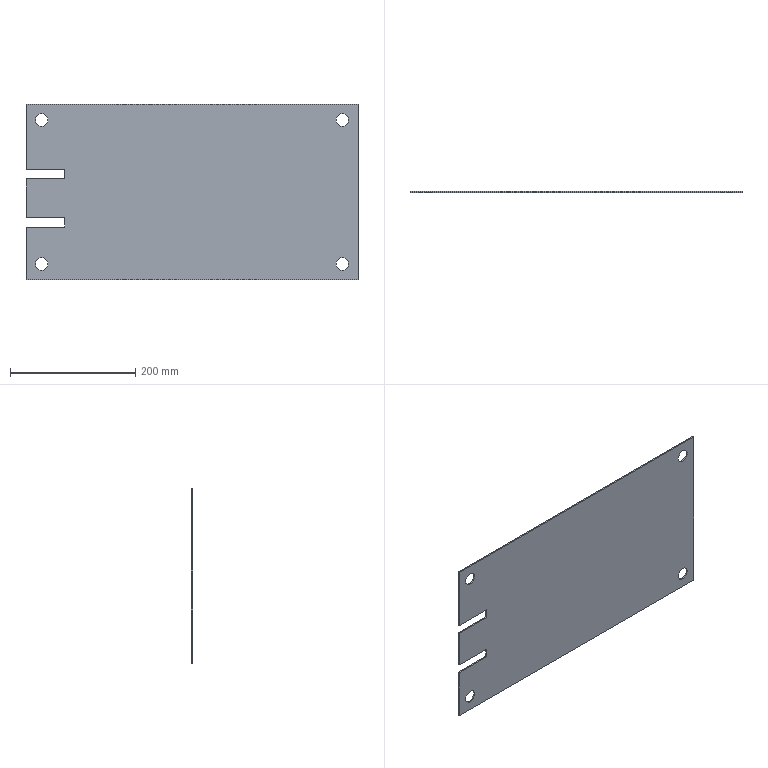Part | SolidWorks | features ICE 2, Extrusion 1 | 1 solid | 22 faces | box 530 x 2 x 280 mm | volume 290567 mm3 | plane 14 | cylinder 8 | commonest cylinder face diameters 20 x8
STEP:
#1=CARTESIAN_POINT('',(240.,0.,-125.));
#2=VERTEX_POINT('',#1);
#3=CARTESIAN_POINT('',(240.,0.,-105.));
#4=VERTEX_POINT('',#3);
#5=CARTESIAN_POINT('',(240.,0.,-115.));
#6=DIRECTION('',(0.,1.,0.));
#7=DIRECTION('',(0.,0.,-1.));
#8=AXIS2_PLACEMENT_3D('',#5,#6,#7);
#9=CIRCLE('',#8,10.);
#10=EDGE_CURVE('',#2,#4,#9,.T.);
#11=ORIENTED_EDGE('',*,*,#10,.F.);
#12=CARTESIAN_POINT('',(240.,2.,-125.));
#13=VERTEX_POINT('',#12);
#14=CARTESIAN_POINT('',(240.,0.,-125.));
#15=DIRECTION('',(0.,1.,0.));
#16=VECTOR('',#15,1000.);
#17=LINE('',#14,#16);
#18=EDGE_CURVE('',#2,#13,#17,.T.);
#19=ORIENTED_EDGE('',*,*,#18,.T.);
#20=CARTESIAN_POINT('',(240.,2.,-105.));
#21=VERTEX_POINT('',#20);
#22=CARTESIAN_POINT('',(240.,2.,-115.));
#23=DIRECTION('',(0.,1.,0.));
#24=DIRECTION('',(0.,0.,-1.));
#25=AXIS2_PLACEMENT_3D('',#22,#23,#24);
#26=CIRCLE('',#25,10.);
#27=EDGE_CURVE('',#13,#21,#26,.T.);
#28=ORIENTED_EDGE('',*,*,#27,.T.);
#29=CARTESIAN_POINT('',(240.,0.,-105.));
#30=DIRECTION('',(0.,1.,0.));
#31=VECTOR('',#30,1000.);
#32=LINE('',#29,#31);
#33=EDGE_CURVE('',#4,#21,#32,.T.);
#34=ORIENTED_EDGE('',*,*,#33,.F.);
#35=EDGE_LOOP('',(#11,#19,#28,#34));
#36=FACE_OUTER_BOUND('',#35,.T.);
#37=CARTESIAN_POINT('',(240.,0.,-115.));
#38=DIRECTION('',(0.,1.,0.));
#39=DIRECTION('',(0.,0.,1.));
#40=AXIS2_PLACEMENT_3D('',#37,#38,#39);
#41=CYLINDRICAL_SURFACE('',#40,10.);
#42=ADVANCED_FACE('',(#36),#41,.F.);
#43=CARTESIAN_POINT('',(240.,0.,105.));
#44=VERTEX_POINT('',#43);
#45=CARTESIAN_POINT('',(240.,0.,125.));
#46=VERTEX_POINT('',#45);
#47=CARTESIAN_POINT('',(240.,0.,115.));
#48=DIRECTION('',(0.,1.,0.));
#49=DIRECTION('',(0.,0.,1.));
#50=AXIS2_PLACEMENT_3D('',#47,#48,#49);
#51=CIRCLE('',#50,10.);
#52=EDGE_CURVE('',#44,#46,#51,.T.);
#53=ORIENTED_EDGE('',*,*,#52,.F.);
#54=CARTESIAN_POINT('',(240.,2.,105.));
#55=VERTEX_POINT('',#54);
#56=CARTESIAN_POINT('',(240.,0.,105.));
#57=DIRECTION('',(0.,1.,0.));
#58=VECTOR('',#57,1000.);
#59=LINE('',#56,#58);
#60=EDGE_CURVE('',#44,#55,#59,.T.);
#61=ORIENTED_EDGE('',*,*,#60,.T.);
#62=CARTESIAN_POINT('',(240.,2.,125.));
#63=VERTEX_POINT('',#62);
#64=CARTESIAN_POINT('',(240.,2.,115.));
#65=DIRECTION('',(0.,1.,0.));
#66=DIRECTION('',(0.,0.,1.));
#67=AXIS2_PLACEMENT_3D('',#64,#65,#66);
#68=CIRCLE('',#67,10.);
#69=EDGE_CURVE('',#55,#63,#68,.T.);
#70=ORIENTED_EDGE('',*,*,#69,.T.);
#71=CARTESIAN_POINT('',(240.,0.,125.));
#72=DIRECTION('',(0.,1.,0.));
#73=VECTOR('',#72,1000.);
#74=LINE('',#71,#73);
#75=EDGE_CURVE('',#46,#63,#74,.T.);
#76=ORIENTED_EDGE('',*,*,#75,.F.);
#77=EDGE_LOOP('',(#53,#61,#70,#76));
#78=FACE_OUTER_BOUND('',#77,.T.);
#79=CARTESIAN_POINT('',(240.,0.,115.));
#80=DIRECTION('',(0.,1.,0.));
#81=DIRECTION('',(0.,0.,1.));
#82=AXIS2_PLACEMENT_3D('',#79,#80,#81);
#83=CYLINDRICAL_SURFACE('',#82,10.);
#84=ADVANCED_FACE('',(#78),#83,.F.);
#85=CARTESIAN_POINT('',(-240.,0.,105.));
#86=VERTEX_POINT('',#85);
#87=CARTESIAN_POINT('',(-240.,0.,125.));
#88=VERTEX_POINT('',#87);
#89=CARTESIAN_POINT('',(-240.,0.,115.));
#90=DIRECTION('',(0.,1.,0.));
#91=DIRECTION('',(0.,0.,-1.));
#92=AXIS2_PLACEMENT_3D('',#89,#90,#91);
#93=CIRCLE('',#92,10.);
#94=EDGE_CURVE('',#86,#88,#93,.T.);
#95=ORIENTED_EDGE('',*,*,#94,.F.);
#96=CARTESIAN_POINT('',(-240.,2.,105.));
#97=VERTEX_POINT('',#96);
#98=CARTESIAN_POINT('',(-240.,0.,105.));
#99=DIRECTION('',(0.,1.,0.));
#100=VECTOR('',#99,1000.);
#101=LINE('',#98,#100);
#102=EDGE_CURVE('',#86,#97,#101,.T.);
#103=ORIENTED_EDGE('',*,*,#102,.T.);
#104=CARTESIAN_POINT('',(-240.,2.,125.));
#105=VERTEX_POINT('',#104);
#106=CARTESIAN_POINT('',(-240.,2.,115.));
#107=DIRECTION('',(0.,1.,0.));
#108=DIRECTION('',(0.,0.,-1.));
#109=AXIS2_PLACEMENT_3D('',#106,#107,#108);
#110=CIRCLE('',#109,10.);
#111=EDGE_CURVE('',#97,#105,#110,.T.);
#112=ORIENTED_EDGE('',*,*,#111,.T.);
#113=CARTESIAN_POINT('',(-240.,0.,125.));
#114=DIRECTION('',(0.,1.,0.));
#115=VECTOR('',#114,1000.);
#116=LINE('',#113,#115);
#117=EDGE_CURVE('',#88,#105,#116,.T.);
#118=ORIENTED_EDGE('',*,*,#117,.F.);
#119=EDGE_LOOP('',(#95,#103,#112,#118));
#120=FACE_OUTER_BOUND('',#119,.T.);
#121=CARTESIAN_POINT('',(-240.,0.,115.));
#122=DIRECTION('',(0.,1.,0.));
#123=DIRECTION('',(0.,0.,1.));
#124=AXIS2_PLACEMENT_3D('',#121,#122,#123);
#125=CYLINDRICAL_SURFACE('',#124,10.);
#126=ADVANCED_FACE('',(#120),#125,.F.);
#127=CARTESIAN_POINT('',(-240.,0.,-125.));
#128=VERTEX_POINT('',#127);
#129=CARTESIAN_POINT('',(-240.,0.,-105.));
#130=VERTEX_POINT('',#129);
#131=CARTESIAN_POINT('',(-240.,0.,-115.));
#132=DIRECTION('',(0.,1.,0.));
#133=DIRECTION('',(0.,0.,1.));
#134=AXIS2_PLACEMENT_3D('',#131,#132,#133);
#135=CIRCLE('',#134,10.);
#136=EDGE_CURVE('',#128,#130,#135,.T.);
#137=ORIENTED_EDGE('',*,*,#136,.F.);
#138=CARTESIAN_POINT('',(-240.,2.,-125.));
#139=VERTEX_POINT('',#138);
#140=CARTESIAN_POINT('',(-240.,0.,-125.));
#141=DIRECTION('',(0.,1.,0.));
#142=VECTOR('',#141,1000.);
#143=LINE('',#140,#142);
#144=EDGE_CURVE('',#128,#139,#143,.T.);
#145=ORIENTED_EDGE('',*,*,#144,.T.);
#146=CARTESIAN_POINT('',(-240.,2.,-105.));
#147=VERTEX_POINT('',#146);
#148=CARTESIAN_POINT('',(-240.,2.,-115.));
#149=DIRECTION('',(0.,1.,0.));
#150=DIRECTION('',(0.,0.,1.));
#151=AXIS2_PLACEMENT_3D('',#148,#149,#150);
#152=CIRCLE('',#151,10.);
#153=EDGE_CURVE('',#139,#147,#152,.T.);
#154=ORIENTED_EDGE('',*,*,#153,.T.);
#155=CARTESIAN_POINT('',(-240.,0.,-105.));
#156=DIRECTION('',(0.,1.,0.));
#157=VECTOR('',#156,1000.);
#158=LINE('',#155,#157);
#159=EDGE_CURVE('',#130,#147,#158,.T.);
#160=ORIENTED_EDGE('',*,*,#159,.F.);
#161=EDGE_LOOP('',(#137,#145,#154,#160));
#162=FACE_OUTER_BOUND('',#161,.T.);
#163=CARTESIAN_POINT('',(-240.,0.,-115.));
#164=DIRECTION('',(0.,1.,0.));
#165=DIRECTION('',(0.,0.,1.));
#166=AXIS2_PLACEMENT_3D('',#163,#164,#165);
#167=CYLINDRICAL_SURFACE('',#166,10.);
#168=ADVANCED_FACE('',(#162),#167,.F.);
#169=CARTESIAN_POINT('',(-265.,0.,-41.));
#170=VERTEX_POINT('',#169);
#171=CARTESIAN_POINT('',(-265.,0.,21.));
#172=VERTEX_POINT('',#171);
#173=CARTESIAN_POINT('',(-265.,0.,140.));
#174=DIRECTION('',(0.,0.,1.));
#175=VECTOR('',#174,1000.);
#176=LINE('',#173,#175);
#177=EDGE_CURVE('',#170,#172,#176,.T.);
#178=ORIENTED_EDGE('',*,*,#177,.T.);
#179=CARTESIAN_POINT('',(-265.,2.,21.));
#180=VERTEX_POINT('',#179);
#181=CARTESIAN_POINT('',(-265.,2.,21.));
#182=DIRECTION('',(0.,1.,0.));
#183=VECTOR('',#182,1000.);
#184=LINE('',#181,#183);
#185=EDGE_CURVE('',#172,#180,#184,.T.);
#186=ORIENTED_EDGE('',*,*,#185,.T.);
#187=CARTESIAN_POINT('',(-265.,2.,-41.));
#188=VERTEX_POINT('',#187);
#189=CARTESIAN_POINT('',(-265.,2.,140.));
#190=DIRECTION('',(0.,0.,1.));
#191=VECTOR('',#190,1000.);
#192=LINE('',#189,#191);
#193=EDGE_CURVE('',#188,#180,#192,.T.);
#194=ORIENTED_EDGE('',*,*,#193,.F.);
#195=CARTESIAN_POINT('',(-265.,2.,-41.));
#196=DIRECTION('',(0.,-1.,0.));
#197=VECTOR('',#196,1000.);
#198=LINE('',#195,#197);
#199=EDGE_CURVE('',#188,#170,#198,.T.);
#200=ORIENTED_EDGE('',*,*,#199,.T.);
#201=EDGE_LOOP('',(#178,#186,#194,#200));
#202=FACE_OUTER_BOUND('',#201,.T.);
#203=CARTESIAN_POINT('',(-265.,2.,140.));
#204=DIRECTION('',(1.,0.,0.));
#205=DIRECTION('',(0.,0.,-1.));
#206=AXIS2_PLACEMENT_3D('',#203,#204,#205);
#207=PLANE('',#206);
#208=ADVANCED_FACE('',(#202),#207,.F.);
#209=CARTESIAN_POINT('',(-265.,0.,-140.));
#210=VERTEX_POINT('',#209);
#211=CARTESIAN_POINT('',(-265.,0.,-56.));
#212=VERTEX_POINT('',#211);
#213=CARTESIAN_POINT('',(-265.,0.,140.));
#214=DIRECTION('',(0.,0.,1.));
#215=VECTOR('',#214,1000.);
#216=LINE('',#213,#215);
#217=EDGE_CURVE('',#210,#212,#216,.T.);
#218=ORIENTED_EDGE('',*,*,#217,.T.);
#219=CARTESIAN_POINT('',(-265.,2.,-56.));
#220=VERTEX_POINT('',#219);
#221=CARTESIAN_POINT('',(-265.,2.,-56.));
#222=DIRECTION('',(0.,1.,0.));
#223=VECTOR('',#222,1000.);
#224=LINE('',#221,#223);
#225=EDGE_CURVE('',#212,#220,#224,.T.);
#226=ORIENTED_EDGE('',*,*,#225,.T.);
#227=CARTESIAN_POINT('',(-265.,2.,-140.));
#228=VERTEX_POINT('',#227);
#229=CARTESIAN_POINT('',(-265.,2.,140.));
#230=DIRECTION('',(0.,0.,1.));
#231=VECTOR('',#230,1000.);
#232=LINE('',#229,#231);
#233=EDGE_CURVE('',#228,#220,#232,.T.);
#234=ORIENTED_EDGE('',*,*,#233,.F.);
#235=CARTESIAN_POINT('',(-265.,2.,-140.));
#236=DIRECTION('',(0.,-1.,0.));
#237=VECTOR('',#236,1000.);
#238=LINE('',#235,#237);
#239=EDGE_CURVE('',#228,#210,#238,.T.);
#240=ORIENTED_EDGE('',*,*,#239,.T.);
#241=EDGE_LOOP('',(#218,#226,#234,#240));
#242=FACE_OUTER_BOUND('',#241,.T.);
#243=CARTESIAN_POINT('',(-265.,2.,140.));
#244=DIRECTION('',(1.,0.,0.));
#245=DIRECTION('',(0.,0.,-1.));
#246=AXIS2_PLACEMENT_3D('',#243,#244,#245);
#247=PLANE('',#246);
#248=ADVANCED_FACE('',(#242),#247,.F.);
#249=CARTESIAN_POINT('',(265.,0.,140.));
#250=VERTEX_POINT('',#249);
#251=CARTESIAN_POINT('',(265.,0.,-140.));
#252=VERTEX_POINT('',#251);
#253=CARTESIAN_POINT('',(265.,0.,140.));
#254=DIRECTION('',(0.,0.,-1.));
#255=VECTOR('',#254,1000.);
#256=LINE('',#253,#255);
#257=EDGE_CURVE('',#250,#252,#256,.T.);
#258=ORIENTED_EDGE('',*,*,#257,.T.);
#259=CARTESIAN_POINT('',(265.,2.,-140.));
#260=VERTEX_POINT('',#259);
#261=CARTESIAN_POINT('',(265.,2.,-140.));
#262=DIRECTION('',(0.,-1.,0.));
#263=VECTOR('',#262,1000.);
#264=LINE('',#261,#263);
#265=EDGE_CURVE('',#260,#252,#264,.T.);
#266=ORIENTED_EDGE('',*,*,#265,.F.);
#267=CARTESIAN_POINT('',(265.,2.,140.));
#268=VERTEX_POINT('',#267);
#269=CARTESIAN_POINT('',(265.,2.,140.));
#270=DIRECTION('',(0.,0.,-1.));
#271=VECTOR('',#270,1000.);
#272=LINE('',#269,#271);
#273=EDGE_CURVE('',#268,#260,#272,.T.);
#274=ORIENTED_EDGE('',*,*,#273,.F.);
#275=CARTESIAN_POINT('',(265.,2.,140.));
#276=DIRECTION('',(0.,-1.,0.));
#277=VECTOR('',#276,1000.);
#278=LINE('',#275,#277);
#279=EDGE_CURVE('',#268,#250,#278,.T.);
#280=ORIENTED_EDGE('',*,*,#279,.T.);
#281=EDGE_LOOP('',(#258,#266,#274,#280));
#282=FACE_OUTER_BOUND('',#281,.T.);
#283=CARTESIAN_POINT('',(265.,2.,140.));
#284=DIRECTION('',(-1.,0.,0.));
#285=DIRECTION('',(0.,0.,1.));
#286=AXIS2_PLACEMENT_3D('',#283,#284,#285);
#287=PLANE('',#286);
#288=ADVANCED_FACE('',(#282),#287,.F.);
#289=CARTESIAN_POINT('',(-265.,0.,-140.));
#290=DIRECTION('',(-1.,0.,0.));
#291=VECTOR('',#290,1000.);
#292=LINE('',#289,#291);
#293=EDGE_CURVE('',#252,#210,#292,.T.);
#294=ORIENTED_EDGE('',*,*,#293,.T.);
#295=ORIENTED_EDGE('',*,*,#239,.F.);
#296=CARTESIAN_POINT('',(-265.,2.,-140.));
#297=DIRECTION('',(-1.,0.,0.));
#298=VECTOR('',#297,1000.);
#299=LINE('',#296,#298);
#300=EDGE_CURVE('',#260,#228,#299,.T.);
#301=ORIENTED_EDGE('',*,*,#300,.F.);
#302=ORIENTED_EDGE('',*,*,#265,.T.);
#303=EDGE_LOOP('',(#294,#295,#301,#302));
#304=FACE_OUTER_BOUND('',#303,.T.);
#305=CARTESIAN_POINT('',(-265.,2.,-140.));
#306=DIRECTION('',(0.,0.,1.));
#307=DIRECTION('',(1.,0.,0.));
#308=AXIS2_PLACEMENT_3D('',#305,#306,#307);
#309=PLANE('',#308);
#310=ADVANCED_FACE('',(#304),#309,.F.);
#311=CARTESIAN_POINT('',(-265.,2.,36.));
#312=VERTEX_POINT('',#311);
#313=CARTESIAN_POINT('',(-265.,2.,140.));
#314=VERTEX_POINT('',#313);
#315=CARTESIAN_POINT('',(-265.,2.,140.));
#316=DIRECTION('',(0.,0.,1.));
#317=VECTOR('',#316,1000.);
#318=LINE('',#315,#317);
#319=EDGE_CURVE('',#312,#314,#318,.T.);
#320=ORIENTED_EDGE('',*,*,#319,.F.);
#321=CARTESIAN_POINT('',(-265.,0.,36.));
#322=VERTEX_POINT('',#321);
#323=CARTESIAN_POINT('',(-265.,2.,36.));
#324=DIRECTION('',(0.,-1.,0.));
#325=VECTOR('',#324,1000.);
#326=LINE('',#323,#325);
#327=EDGE_CURVE('',#312,#322,#326,.T.);
#328=ORIENTED_EDGE('',*,*,#327,.T.);
#329=CARTESIAN_POINT('',(-265.,0.,140.));
#330=VERTEX_POINT('',#329);
#331=CARTESIAN_POINT('',(-265.,0.,140.));
#332=DIRECTION('',(0.,0.,1.));
#333=VECTOR('',#332,1000.);
#334=LINE('',#331,#333);
#335=EDGE_CURVE('',#322,#330,#334,.T.);
#336=ORIENTED_EDGE('',*,*,#335,.T.);
#337=CARTESIAN_POINT('',(-265.,2.,140.));
#338=DIRECTION('',(0.,-1.,0.));
#339=VECTOR('',#338,1000.);
#340=LINE('',#337,#339);
#341=EDGE_CURVE('',#314,#330,#340,.T.);
#342=ORIENTED_EDGE('',*,*,#341,.F.);
#343=EDGE_LOOP('',(#320,#328,#336,#342));
#344=FACE_OUTER_BOUND('',#343,.T.);
#345=CARTESIAN_POINT('',(-265.,2.,140.));
#346=DIRECTION('',(1.,0.,0.));
#347=DIRECTION('',(0.,0.,-1.));
#348=AXIS2_PLACEMENT_3D('',#345,#346,#347);
#349=PLANE('',#348);
#350=ADVANCED_FACE('',(#344),#349,.F.);
#351=CARTESIAN_POINT('',(-265.,0.,140.));
#352=DIRECTION('',(1.,0.,0.));
#353=VECTOR('',#352,1000.);
#354=LINE('',#351,#353);
#355=EDGE_CURVE('',#330,#250,#354,.T.);
#356=ORIENTED_EDGE('',*,*,#355,.T.);
#357=ORIENTED_EDGE('',*,*,#279,.F.);
#358=CARTESIAN_POINT('',(-265.,2.,140.));
#359=DIRECTION('',(1.,0.,0.));
#360=VECTOR('',#359,1000.);
#361=LINE('',#358,#360);
#362=EDGE_CURVE('',#314,#268,#361,.T.);
#363=ORIENTED_EDGE('',*,*,#362,.F.);
#364=ORIENTED_EDGE('',*,*,#341,.T.);
#365=EDGE_LOOP('',(#356,#357,#363,#364));
#366=FACE_OUTER_BOUND('',#365,.T.);
#367=CARTESIAN_POINT('',(-265.,2.,140.));
#368=DIRECTION('',(0.,0.,-1.));
#369=DIRECTION('',(-1.,0.,0.));
#370=AXIS2_PLACEMENT_3D('',#367,#368,#369);
#371=PLANE('',#370);
#372=ADVANCED_FACE('',(#366),#371,.F.);
#373=CARTESIAN_POINT('',(240.,2.,-115.));
#374=DIRECTION('',(0.,1.,0.));
#375=DIRECTION('',(0.,0.,-1.));
#376=AXIS2_PLACEMENT_3D('',#373,#374,#375);
#377=CIRCLE('',#376,10.);
#378=EDGE_CURVE('',#21,#13,#377,.T.);
#379=ORIENTED_EDGE('',*,*,#378,.F.);
#380=ORIENTED_EDGE('',*,*,#27,.F.);
#381=EDGE_LOOP('',(#379,#380));
#382=FACE_BOUND('',#381,.T.);
#383=CARTESIAN_POINT('',(240.,2.,115.));
#384=DIRECTION('',(0.,1.,0.));
#385=DIRECTION('',(0.,0.,1.));
#386=AXIS2_PLACEMENT_3D('',#383,#384,#385);
#387=CIRCLE('',#386,10.);
#388=EDGE_CURVE('',#63,#55,#387,.T.);
#389=ORIENTED_EDGE('',*,*,#388,.F.);
#390=ORIENTED_EDGE('',*,*,#69,.F.);
#391=EDGE_LOOP('',(#389,#390));
#392=FACE_BOUND('',#391,.T.);
#393=CARTESIAN_POINT('',(-240.,2.,115.));
#394=DIRECTION('',(0.,1.,0.));
#395=DIRECTION('',(0.,0.,-1.));
#396=AXIS2_PLACEMENT_3D('',#393,#394,#395);
#397=CIRCLE('',#396,10.);
#398=EDGE_CURVE('',#105,#97,#397,.T.);
#399=ORIENTED_EDGE('',*,*,#398,.F.);
#400=ORIENTED_EDGE('',*,*,#111,.F.);
#401=EDGE_LOOP('',(#399,#400));
#402=FACE_BOUND('',#401,.T.);
#403=CARTESIAN_POINT('',(-240.,2.,-115.));
#404=DIRECTION('',(0.,1.,0.));
#405=DIRECTION('',(0.,0.,1.));
#406=AXIS2_PLACEMENT_3D('',#403,#404,#405);
#407=CIRCLE('',#406,10.);
#408=EDGE_CURVE('',#147,#139,#407,.T.);
#409=ORIENTED_EDGE('',*,*,#408,.F.);
#410=ORIENTED_EDGE('',*,*,#153,.F.);
#411=EDGE_LOOP('',(#409,#410));
#412=FACE_BOUND('',#411,.T.);
#413=ORIENTED_EDGE('',*,*,#193,.T.);
#414=CARTESIAN_POINT('',(-203.,2.,21.));
#415=VERTEX_POINT('',#414);
#416=CARTESIAN_POINT('',(-299.084,2.,21.));
#417=DIRECTION('',(-1.,0.,0.));
#418=VECTOR('',#417,1000.);
#419=LINE('',#416,#418);
#420=EDGE_CURVE('',#415,#180,#419,.T.);
#421=ORIENTED_EDGE('',*,*,#420,.F.);
#422=CARTESIAN_POINT('',(-203.,2.,36.));
#423=VERTEX_POINT('',#422);
#424=CARTESIAN_POINT('',(-203.,2.,21.));
#425=DIRECTION('',(0.,0.,-1.));
#426=VECTOR('',#425,1000.);
#427=LINE('',#424,#426);
#428=EDGE_CURVE('',#423,#415,#427,.T.);
#429=ORIENTED_EDGE('',*,*,#428,.F.);
#430=CARTESIAN_POINT('',(-299.084,2.,36.));
#431=DIRECTION('',(1.,0.,0.));
#432=VECTOR('',#431,1000.);
#433=LINE('',#430,#432);
#434=EDGE_CURVE('',#312,#423,#433,.T.);
#435=ORIENTED_EDGE('',*,*,#434,.F.);
#436=ORIENTED_EDGE('',*,*,#319,.T.);
#437=ORIENTED_EDGE('',*,*,#362,.T.);
#438=ORIENTED_EDGE('',*,*,#273,.T.);
#439=ORIENTED_EDGE('',*,*,#300,.T.);
#440=ORIENTED_EDGE('',*,*,#233,.T.);
#441=CARTESIAN_POINT('',(-203.,2.,-56.));
#442=VERTEX_POINT('',#441);
#443=CARTESIAN_POINT('',(-296.313,2.,-56.));
#444=DIRECTION('',(-1.,0.,0.));
#445=VECTOR('',#444,1000.);
#446=LINE('',#443,#445);
#447=EDGE_CURVE('',#442,#220,#446,.T.);
#448=ORIENTED_EDGE('',*,*,#447,.F.);
#449=CARTESIAN_POINT('',(-203.,2.,-41.));
#450=VERTEX_POINT('',#449);
#451=CARTESIAN_POINT('',(-203.,2.,-56.));
#452=DIRECTION('',(0.,0.,-1.));
#453=VECTOR('',#452,1000.);
#454=LINE('',#451,#453);
#455=EDGE_CURVE('',#450,#442,#454,.T.);
#456=ORIENTED_EDGE('',*,*,#455,.F.);
#457=CARTESIAN_POINT('',(-296.313,2.,-41.));
#458=DIRECTION('',(1.,0.,0.));
#459=VECTOR('',#458,1000.);
#460=LINE('',#457,#459);
#461=EDGE_CURVE('',#188,#450,#460,.T.);
#462=ORIENTED_EDGE('',*,*,#461,.F.);
#463=EDGE_LOOP('',(#413,#421,#429,#435,#436,#437,#438,#439,#440,#448,#456,#462));
#464=FACE_OUTER_BOUND('',#463,.T.);
#465=CARTESIAN_POINT('',(0.,2.,0.));
#466=DIRECTION('',(0.,-1.,0.));
#467=DIRECTION('',(0.,0.,-1.));
#468=AXIS2_PLACEMENT_3D('',#465,#466,#467);
#469=PLANE('',#468);
#470=ADVANCED_FACE('',(#382,#392,#402,#412,#464),#469,.F.);
#471=CARTESIAN_POINT('',(-203.,0.,21.));
#472=VERTEX_POINT('',#471);
#473=CARTESIAN_POINT('',(0.,0.,21.));
#474=DIRECTION('',(1.,0.,0.));
#475=VECTOR('',#474,1000.);
#476=LINE('',#473,#475);
#477=EDGE_CURVE('',#172,#472,#476,.T.);
#478=ORIENTED_EDGE('',*,*,#477,.F.);
#479=ORIENTED_EDGE('',*,*,#177,.F.);
#480=CARTESIAN_POINT('',(-203.,0.,-41.));
#481=VERTEX_POINT('',#480);
#482=CARTESIAN_POINT('',(0.,0.,-41.));
#483=DIRECTION('',(-1.,0.,0.));
#484=VECTOR('',#483,1000.);
#485=LINE('',#482,#484);
#486=EDGE_CURVE('',#481,#170,#485,.T.);
#487=ORIENTED_EDGE('',*,*,#486,.F.);
#488=CARTESIAN_POINT('',(-203.,0.,-56.));
#489=VERTEX_POINT('',#488);
#490=CARTESIAN_POINT('',(-203.,0.,0.));
#491=DIRECTION('',(0.,0.,1.));
#492=VECTOR('',#491,1000.);
#493=LINE('',#490,#492);
#494=EDGE_CURVE('',#489,#481,#493,.T.);
#495=ORIENTED_EDGE('',*,*,#494,.F.);
#496=CARTESIAN_POINT('',(0.,0.,-56.));
#497=DIRECTION('',(1.,0.,0.));
#498=VECTOR('',#497,1000.);
#499=LINE('',#496,#498);
#500=EDGE_CURVE('',#212,#489,#499,.T.);
#501=ORIENTED_EDGE('',*,*,#500,.F.);
#502=ORIENTED_EDGE('',*,*,#217,.F.);
#503=ORIENTED_EDGE('',*,*,#293,.F.);
#504=ORIENTED_EDGE('',*,*,#257,.F.);
#505=ORIENTED_EDGE('',*,*,#355,.F.);
#506=ORIENTED_EDGE('',*,*,#335,.F.);
#507=CARTESIAN_POINT('',(-203.,0.,36.));
#508=VERTEX_POINT('',#507);
#509=CARTESIAN_POINT('',(0.,0.,36.));
#510=DIRECTION('',(-1.,0.,0.));
#511=VECTOR('',#510,1000.);
#512=LINE('',#509,#511);
#513=EDGE_CURVE('',#508,#322,#512,.T.);
#514=ORIENTED_EDGE('',*,*,#513,.F.);
#515=CARTESIAN_POINT('',(-203.,0.,0.));
#516=DIRECTION('',(0.,0.,1.));
#517=VECTOR('',#516,1000.);
#518=LINE('',#515,#517);
#519=EDGE_CURVE('',#472,#508,#518,.T.);
#520=ORIENTED_EDGE('',*,*,#519,.F.);
#521=EDGE_LOOP('',(#478,#479,#487,#495,#501,#502,#503,#504,#505,#506,#514,#520));
#522=FACE_OUTER_BOUND('',#521,.T.);
#523=CARTESIAN_POINT('',(240.,0.,-115.));
#524=DIRECTION('',(0.,1.,0.));
#525=DIRECTION('',(0.,0.,-1.));
#526=AXIS2_PLACEMENT_3D('',#523,#524,#525);
#527=CIRCLE('',#526,10.);
#528=EDGE_CURVE('',#4,#2,#527,.T.);
#529=ORIENTED_EDGE('',*,*,#528,.T.);
#530=ORIENTED_EDGE('',*,*,#10,.T.);
#531=EDGE_LOOP('',(#529,#530));
#532=FACE_BOUND('',#531,.T.);
#533=CARTESIAN_POINT('',(240.,0.,115.));
#534=DIRECTION('',(0.,1.,0.));
#535=DIRECTION('',(0.,0.,1.));
#536=AXIS2_PLACEMENT_3D('',#533,#534,#535);
#537=CIRCLE('',#536,10.);
#538=EDGE_CURVE('',#46,#44,#537,.T.);
#539=ORIENTED_EDGE('',*,*,#538,.T.);
#540=ORIENTED_EDGE('',*,*,#52,.T.);
#541=EDGE_LOOP('',(#539,#540));
#542=FACE_BOUND('',#541,.T.);
#543=CARTESIAN_POINT('',(-240.,0.,115.));
#544=DIRECTION('',(0.,1.,0.));
#545=DIRECTION('',(0.,0.,-1.));
#546=AXIS2_PLACEMENT_3D('',#543,#544,#545);
#547=CIRCLE('',#546,10.);
#548=EDGE_CURVE('',#88,#86,#547,.T.);
#549=ORIENTED_EDGE('',*,*,#548,.T.);
#550=ORIENTED_EDGE('',*,*,#94,.T.);
#551=EDGE_LOOP('',(#549,#550));
#552=FACE_BOUND('',#551,.T.);
#553=CARTESIAN_POINT('',(-240.,0.,-115.));
#554=DIRECTION('',(0.,1.,0.));
#555=DIRECTION('',(0.,0.,1.));
#556=AXIS2_PLACEMENT_3D('',#553,#554,#555);
#557=CIRCLE('',#556,10.);
#558=EDGE_CURVE('',#130,#128,#557,.T.);
#559=ORIENTED_EDGE('',*,*,#558,.T.);
#560=ORIENTED_EDGE('',*,*,#136,.T.);
#561=EDGE_LOOP('',(#559,#560));
#562=FACE_BOUND('',#561,.T.);
#563=CARTESIAN_POINT('',(0.,0.,0.));
#564=DIRECTION('',(0.,-1.,0.));
#565=DIRECTION('',(0.,0.,-1.));
#566=AXIS2_PLACEMENT_3D('',#563,#564,#565);
#567=PLANE('',#566);
#568=ADVANCED_FACE('',(#522,#532,#542,#552,#562),#567,.T.);
#569=ORIENTED_EDGE('',*,*,#144,.F.);
#570=ORIENTED_EDGE('',*,*,#558,.F.);
#571=ORIENTED_EDGE('',*,*,#159,.T.);
#572=ORIENTED_EDGE('',*,*,#408,.T.);
#573=EDGE_LOOP('',(#569,#570,#571,#572));
#574=FACE_OUTER_BOUND('',#573,.T.);
#575=CARTESIAN_POINT('',(-240.,0.,-115.));
#576=DIRECTION('',(0.,1.,0.));
#577=DIRECTION('',(0.,0.,1.));
#578=AXIS2_PLACEMENT_3D('',#575,#576,#577);
#579=CYLINDRICAL_SURFACE('',#578,10.);
#580=ADVANCED_FACE('',(#574),#579,.F.);
#581=ORIENTED_EDGE('',*,*,#102,.F.);
#582=ORIENTED_EDGE('',*,*,#548,.F.);
#583=ORIENTED_EDGE('',*,*,#117,.T.);
#584=ORIENTED_EDGE('',*,*,#398,.T.);
#585=EDGE_LOOP('',(#581,#582,#583,#584));
#586=FACE_OUTER_BOUND('',#585,.T.);
#587=CARTESIAN_POINT('',(-240.,0.,115.));
#588=DIRECTION('',(0.,1.,0.));
#589=DIRECTION('',(0.,0.,1.));
#590=AXIS2_PLACEMENT_3D('',#587,#588,#589);
#591=CYLINDRICAL_SURFACE('',#590,10.);
#592=ADVANCED_FACE('',(#586),#591,.F.);
#593=ORIENTED_EDGE('',*,*,#60,.F.);
#594=ORIENTED_EDGE('',*,*,#538,.F.);
#595=ORIENTED_EDGE('',*,*,#75,.T.);
#596=ORIENTED_EDGE('',*,*,#388,.T.);
#597=EDGE_LOOP('',(#593,#594,#595,#596));
#598=FACE_OUTER_BOUND('',#597,.T.);
#599=CARTESIAN_POINT('',(240.,0.,115.));
#600=DIRECTION('',(0.,1.,0.));
#601=DIRECTION('',(0.,0.,1.));
#602=AXIS2_PLACEMENT_3D('',#599,#600,#601);
#603=CYLINDRICAL_SURFACE('',#602,10.);
#604=ADVANCED_FACE('',(#598),#603,.F.);
#605=ORIENTED_EDGE('',*,*,#18,.F.);
#606=ORIENTED_EDGE('',*,*,#528,.F.);
#607=ORIENTED_EDGE('',*,*,#33,.T.);
#608=ORIENTED_EDGE('',*,*,#378,.T.);
#609=EDGE_LOOP('',(#605,#606,#607,#608));
#610=FACE_OUTER_BOUND('',#609,.T.);
#611=CARTESIAN_POINT('',(240.,0.,-115.));
#612=DIRECTION('',(0.,1.,0.));
#613=DIRECTION('',(0.,0.,1.));
#614=AXIS2_PLACEMENT_3D('',#611,#612,#613);
#615=CYLINDRICAL_SURFACE('',#614,10.);
#616=ADVANCED_FACE('',(#610),#615,.F.);
#617=ORIENTED_EDGE('',*,*,#500,.T.);
#618=CARTESIAN_POINT('',(-203.,-8.,-56.));
#619=DIRECTION('',(0.,1.,0.));
#620=VECTOR('',#619,1000.);
#621=LINE('',#618,#620);
#622=EDGE_CURVE('',#489,#442,#621,.T.);
#623=ORIENTED_EDGE('',*,*,#622,.T.);
#624=ORIENTED_EDGE('',*,*,#447,.T.);
#625=ORIENTED_EDGE('',*,*,#225,.F.);
#626=EDGE_LOOP('',(#617,#623,#624,#625));
#627=FACE_OUTER_BOUND('',#626,.T.);
#628=CARTESIAN_POINT('',(-296.313,-8.,-56.));
#629=DIRECTION('',(0.,0.,-1.));
#630=DIRECTION('',(-1.,0.,0.));
#631=AXIS2_PLACEMENT_3D('',#628,#629,#630);
#632=PLANE('',#631);
#633=ADVANCED_FACE('',(#627),#632,.F.);
#634=ORIENTED_EDGE('',*,*,#461,.T.);
#635=CARTESIAN_POINT('',(-203.,-8.,-41.));
#636=DIRECTION('',(0.,1.,0.));
#637=VECTOR('',#636,1000.);
#638=LINE('',#635,#637);
#639=EDGE_CURVE('',#481,#450,#638,.T.);
#640=ORIENTED_EDGE('',*,*,#639,.F.);
#641=ORIENTED_EDGE('',*,*,#486,.T.);
#642=ORIENTED_EDGE('',*,*,#199,.F.);
#643=EDGE_LOOP('',(#634,#640,#641,#642));
#644=FACE_OUTER_BOUND('',#643,.T.);
#645=CARTESIAN_POINT('',(-296.313,-8.,-41.));
#646=DIRECTION('',(0.,0.,1.));
#647=DIRECTION('',(1.,0.,0.));
#648=AXIS2_PLACEMENT_3D('',#645,#646,#647);
#649=PLANE('',#648);
#650=ADVANCED_FACE('',(#644),#649,.F.);
#651=ORIENTED_EDGE('',*,*,#494,.T.);
#652=ORIENTED_EDGE('',*,*,#639,.T.);
#653=ORIENTED_EDGE('',*,*,#455,.T.);
#654=ORIENTED_EDGE('',*,*,#622,.F.);
#655=EDGE_LOOP('',(#651,#652,#653,#654));
#656=FACE_OUTER_BOUND('',#655,.T.);
#657=CARTESIAN_POINT('',(-203.,-8.,-56.));
#658=DIRECTION('',(1.,0.,0.));
#659=DIRECTION('',(0.,0.,-1.));
#660=AXIS2_PLACEMENT_3D('',#657,#658,#659);
#661=PLANE('',#660);
#662=ADVANCED_FACE('',(#656),#661,.F.);
#663=ORIENTED_EDGE('',*,*,#477,.T.);
#664=CARTESIAN_POINT('',(-203.,-8.,21.));
#665=DIRECTION('',(0.,1.,0.));
#666=VECTOR('',#665,1000.);
#667=LINE('',#664,#666);
#668=EDGE_CURVE('',#472,#415,#667,.T.);
#669=ORIENTED_EDGE('',*,*,#668,.T.);
#670=ORIENTED_EDGE('',*,*,#420,.T.);
#671=ORIENTED_EDGE('',*,*,#185,.F.);
#672=EDGE_LOOP('',(#663,#669,#670,#671));
#673=FACE_OUTER_BOUND('',#672,.T.);
#674=CARTESIAN_POINT('',(-299.084,-8.,21.));
#675=DIRECTION('',(0.,0.,-1.));
#676=DIRECTION('',(-1.,0.,0.));
#677=AXIS2_PLACEMENT_3D('',#674,#675,#676);
#678=PLANE('',#677);
#679=ADVANCED_FACE('',(#673),#678,.F.);
#680=ORIENTED_EDGE('',*,*,#434,.T.);
#681=CARTESIAN_POINT('',(-203.,-8.,36.));
#682=DIRECTION('',(0.,1.,0.));
#683=VECTOR('',#682,1000.);
#684=LINE('',#681,#683);
#685=EDGE_CURVE('',#508,#423,#684,.T.);
#686=ORIENTED_EDGE('',*,*,#685,.F.);
#687=ORIENTED_EDGE('',*,*,#513,.T.);
#688=ORIENTED_EDGE('',*,*,#327,.F.);
#689=EDGE_LOOP('',(#680,#686,#687,#688));
#690=FACE_OUTER_BOUND('',#689,.T.);
#691=CARTESIAN_POINT('',(-299.084,-8.,36.));
#692=DIRECTION('',(0.,0.,1.));
#693=DIRECTION('',(1.,0.,0.));
#694=AXIS2_PLACEMENT_3D('',#691,#692,#693);
#695=PLANE('',#694);
#696=ADVANCED_FACE('',(#690),#695,.F.);
#697=ORIENTED_EDGE('',*,*,#519,.T.);
#698=ORIENTED_EDGE('',*,*,#685,.T.);
#699=ORIENTED_EDGE('',*,*,#428,.T.);
#700=ORIENTED_EDGE('',*,*,#668,.F.);
#701=EDGE_LOOP('',(#697,#698,#699,#700));
#702=FACE_OUTER_BOUND('',#701,.T.);
#703=CARTESIAN_POINT('',(-203.,-8.,21.));
#704=DIRECTION('',(1.,0.,0.));
#705=DIRECTION('',(0.,0.,-1.));
#706=AXIS2_PLACEMENT_3D('',#703,#704,#705);
#707=PLANE('',#706);
#708=ADVANCED_FACE('',(#702),#707,.F.);
#709=CLOSED_SHELL('',(#42,#84,#126,#168,#208,#248,#288,#310,#350,#372,#470,#568,#580,#592,#604,#616,#633,#650,#662,#679,#696,#708));
#710=MANIFOLD_SOLID_BREP('',#709);
#711=CARTESIAN_POINT('',(0.,0.,0.));
#712=DIRECTION('',(0.,0.,1.));
#713=DIRECTION('',(1.,0.,0.));
#714=AXIS2_PLACEMENT_3D('',#711,#712,#713);
#715=(LENGTH_UNIT()NAMED_UNIT(*)SI_UNIT(.MILLI.,.METRE.));
#716=UNCERTAINTY_MEASURE_WITH_UNIT(LENGTH_MEASURE(0.00001),#715,'','');
#717=(NAMED_UNIT(*)PLANE_ANGLE_UNIT()SI_UNIT($,.RADIAN.));
#718=(NAMED_UNIT(*)SI_UNIT($,.STERADIAN.)SOLID_ANGLE_UNIT());
#719=(GEOMETRIC_REPRESENTATION_CONTEXT(3)GLOBAL_UNCERTAINTY_ASSIGNED_CONTEXT((#716))GLOBAL_UNIT_ASSIGNED_CONTEXT((#715,#717,#718))REPRESENTATION_CONTEXT('',''));
#720=ADVANCED_BREP_SHAPE_REPRESENTATION('',(#710,#714),#719);